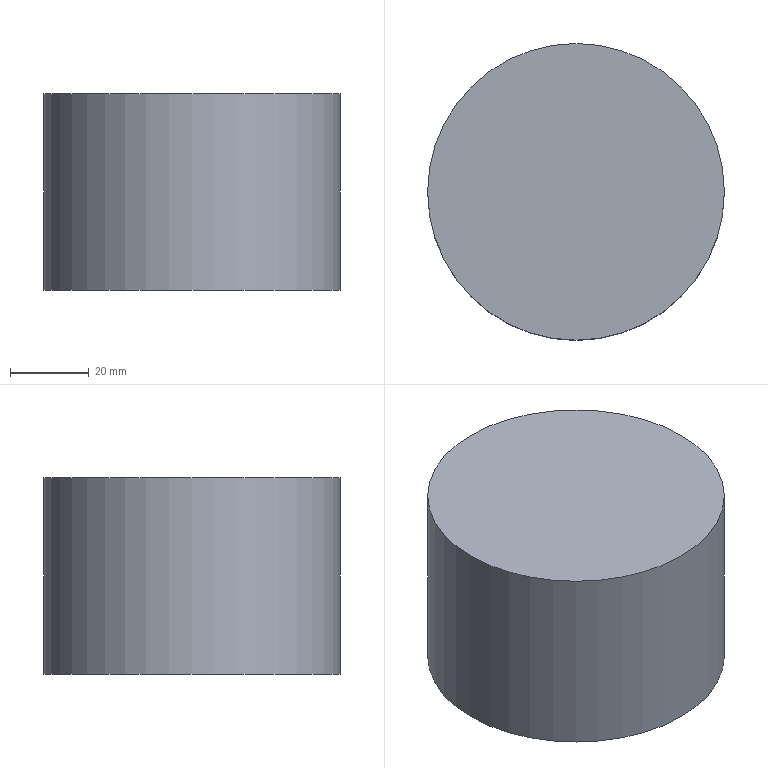Part | NX | features solid 2 | 1 solid | 3 faces | box 75.347 x 75.347 x 50 mm | volume 222939 mm3 | plane 2 | cylinder 1 | commonest cylinder face diameters 75.347 x1
STEP:
#1=CARTESIAN_POINT('',(-1262.327,-300.,-160.));
#2=VERTEX_POINT('',#1);
#3=CARTESIAN_POINT('',(-1300.,-300.,-160.));
#4=DIRECTION('',(0.,0.,1.));
#5=DIRECTION('',(1.,0.,0.));
#6=AXIS2_PLACEMENT_3D('',#3,#4,#5);
#7=CIRCLE('',#6,37.673);
#8=EDGE_CURVE('',#2,#2,#7,.F.);
#9=ORIENTED_EDGE('',*,*,#8,.F.);
#10=EDGE_LOOP('',(#9));
#11=FACE_BOUND('',#10,.T.);
#12=CARTESIAN_POINT('',(-1262.327,-300.,-110.));
#13=VERTEX_POINT('',#12);
#14=CARTESIAN_POINT('',(-1300.,-300.,-110.));
#15=DIRECTION('',(0.,0.,1.));
#16=DIRECTION('',(1.,0.,0.));
#17=AXIS2_PLACEMENT_3D('',#14,#15,#16);
#18=CIRCLE('',#17,37.673);
#19=EDGE_CURVE('',#13,#13,#18,.F.);
#20=ORIENTED_EDGE('',*,*,#19,.T.);
#21=EDGE_LOOP('',(#20));
#22=FACE_BOUND('',#21,.T.);
#23=CARTESIAN_POINT('',(-1300.,-300.,-160.));
#24=DIRECTION('',(0.,0.,1.));
#25=DIRECTION('',(1.,0.,0.));
#26=AXIS2_PLACEMENT_3D('',#23,#24,#25);
#27=CYLINDRICAL_SURFACE('',#26,37.673);
#28=ADVANCED_FACE('',(#11,#22),#27,.T.);
#29=ORIENTED_EDGE('',*,*,#8,.T.);
#30=EDGE_LOOP('',(#29));
#31=FACE_BOUND('',#30,.T.);
#32=CARTESIAN_POINT('',(-1300.,-300.,-160.));
#33=DIRECTION('',(0.,0.,1.));
#34=DIRECTION('',(1.,0.,0.));
#35=AXIS2_PLACEMENT_3D('',#32,#33,#34);
#36=PLANE('',#35);
#37=ADVANCED_FACE('',(#31),#36,.F.);
#38=ORIENTED_EDGE('',*,*,#19,.F.);
#39=EDGE_LOOP('',(#38));
#40=FACE_BOUND('',#39,.T.);
#41=CARTESIAN_POINT('',(-1300.,-300.,-110.));
#42=DIRECTION('',(0.,0.,1.));
#43=DIRECTION('',(1.,0.,0.));
#44=AXIS2_PLACEMENT_3D('',#41,#42,#43);
#45=PLANE('',#44);
#46=ADVANCED_FACE('',(#40),#45,.T.);
#47=CLOSED_SHELL('',(#28,#37,#46));
#48=MANIFOLD_SOLID_BREP('',#47);
#49=(LENGTH_UNIT()NAMED_UNIT(*)SI_UNIT(.MILLI.,.METRE.));
#50=UNCERTAINTY_MEASURE_WITH_UNIT(LENGTH_MEASURE(0.00001),#49,'','');
#51=(NAMED_UNIT(*)PLANE_ANGLE_UNIT()SI_UNIT($,.RADIAN.));
#52=(NAMED_UNIT(*)SI_UNIT($,.STERADIAN.)SOLID_ANGLE_UNIT());
#53=(GEOMETRIC_REPRESENTATION_CONTEXT(3)GLOBAL_UNCERTAINTY_ASSIGNED_CONTEXT((#50))GLOBAL_UNIT_ASSIGNED_CONTEXT((#49,#51,#52))REPRESENTATION_CONTEXT('',''));
#54=ADVANCED_BREP_SHAPE_REPRESENTATION('',(#48),#53);